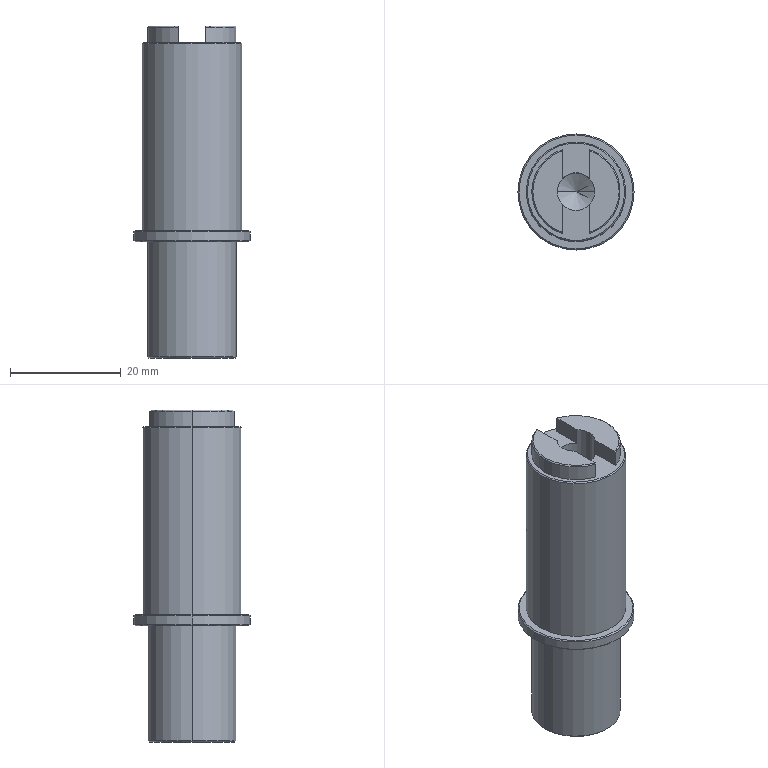Part | SolidWorks | features ICE 4, Chamfer 1, Extrusion 1, HoleWzd 1 | 1 solid | 34 faces | box 21 x 21 x 60 mm | volume 13278 mm3 | cone 13 | cylinder 11 | plane 10 | commonest cylinder face diameters 16 x5 6.8 x2 18 x2 21 x2
STEP:
#1=CARTESIAN_POINT('',(-7.8,0.,37.));
#2=VERTEX_POINT('',#1);
#3=CARTESIAN_POINT('',(-2.5,-7.389,37.));
#4=VERTEX_POINT('',#3);
#5=CARTESIAN_POINT('',(0.,0.,37.));
#6=DIRECTION('',(0.,0.,1.));
#7=DIRECTION('',(1.,0.,0.));
#8=AXIS2_PLACEMENT_3D('',#5,#6,#7);
#9=CIRCLE('',#8,7.8);
#10=EDGE_CURVE('',#2,#4,#9,.T.);
#11=ORIENTED_EDGE('',*,*,#10,.F.);
#12=CARTESIAN_POINT('',(-8.,0.,36.8));
#13=VERTEX_POINT('',#12);
#14=CARTESIAN_POINT('',(-7.8,0.,37.));
#15=DIRECTION('',(-0.7071,0.,-0.7071));
#16=VECTOR('',#15,1000.);
#17=LINE('',#14,#16);
#18=EDGE_CURVE('',#2,#13,#17,.T.);
#19=ORIENTED_EDGE('',*,*,#18,.T.);
#20=CARTESIAN_POINT('',(-2.5,-7.599,36.8));
#21=VERTEX_POINT('',#20);
#22=CARTESIAN_POINT('',(0.,0.,36.8));
#23=DIRECTION('',(0.,0.,-1.));
#24=DIRECTION('',(1.,0.,0.));
#25=AXIS2_PLACEMENT_3D('',#22,#23,#24);
#26=CIRCLE('',#25,8.);
#27=EDGE_CURVE('',#21,#13,#26,.T.);
#28=ORIENTED_EDGE('',*,*,#27,.F.);
#29=CARTESIAN_POINT('',(-2.5,-7.389,37.));
#30=CARTESIAN_POINT('',(-2.5,-7.459,36.933));
#31=CARTESIAN_POINT('',(-2.5,-7.529,36.867));
#32=CARTESIAN_POINT('',(-2.5,-7.599,36.8));
#33=B_SPLINE_CURVE_WITH_KNOTS('',3,(#29,#30,#31,#32),.UNSPECIFIED.,.F.,.F.,(4,4),(0.,0.0002906),.UNSPECIFIED.);
#34=EDGE_CURVE('',#4,#21,#33,.T.);
#35=ORIENTED_EDGE('',*,*,#34,.F.);
#36=EDGE_LOOP('',(#11,#19,#28,#35));
#37=FACE_OUTER_BOUND('',#36,.T.);
#38=CARTESIAN_POINT('',(0.,0.,37.));
#39=DIRECTION('',(0.,0.,-1.));
#40=DIRECTION('',(-1.,0.,0.));
#41=AXIS2_PLACEMENT_3D('',#38,#39,#40);
#42=CONICAL_SURFACE('',#41,7.8,0.7854);
#43=ADVANCED_FACE('',(#37),#42,.T.);
#44=CARTESIAN_POINT('',(8.8,0.,34.));
#45=VERTEX_POINT('',#44);
#46=CARTESIAN_POINT('',(-8.8,0.,34.));
#47=VERTEX_POINT('',#46);
#48=CARTESIAN_POINT('',(0.,0.,34.));
#49=DIRECTION('',(0.,0.,1.));
#50=DIRECTION('',(1.,0.,0.));
#51=AXIS2_PLACEMENT_3D('',#48,#49,#50);
#52=CIRCLE('',#51,8.8);
#53=EDGE_CURVE('',#45,#47,#52,.T.);
#54=ORIENTED_EDGE('',*,*,#53,.F.);
#55=CARTESIAN_POINT('',(9.,0.,33.8));
#56=VERTEX_POINT('',#55);
#57=CARTESIAN_POINT('',(8.8,0.,34.));
#58=DIRECTION('',(0.7071,0.,-0.7071));
#59=VECTOR('',#58,1000.);
#60=LINE('',#57,#59);
#61=EDGE_CURVE('',#45,#56,#60,.T.);
#62=ORIENTED_EDGE('',*,*,#61,.T.);
#63=CARTESIAN_POINT('',(-9.,0.,33.8));
#64=VERTEX_POINT('',#63);
#65=CARTESIAN_POINT('',(0.,0.,33.8));
#66=DIRECTION('',(0.,0.,-1.));
#67=DIRECTION('',(1.,0.,0.));
#68=AXIS2_PLACEMENT_3D('',#65,#66,#67);
#69=CIRCLE('',#68,9.);
#70=EDGE_CURVE('',#64,#56,#69,.T.);
#71=ORIENTED_EDGE('',*,*,#70,.F.);
#72=CARTESIAN_POINT('',(-8.8,0.,34.));
#73=DIRECTION('',(-0.7071,0.,-0.7071));
#74=VECTOR('',#73,1000.);
#75=LINE('',#72,#74);
#76=EDGE_CURVE('',#47,#64,#75,.T.);
#77=ORIENTED_EDGE('',*,*,#76,.F.);
#78=EDGE_LOOP('',(#54,#62,#71,#77));
#79=FACE_OUTER_BOUND('',#78,.T.);
#80=CARTESIAN_POINT('',(0.,0.,34.));
#81=DIRECTION('',(0.,0.,-1.));
#82=DIRECTION('',(-1.,0.,0.));
#83=AXIS2_PLACEMENT_3D('',#80,#81,#82);
#84=CONICAL_SURFACE('',#83,8.8,0.7854);
#85=ADVANCED_FACE('',(#79),#84,.T.);
#86=CARTESIAN_POINT('',(10.3,0.,0.));
#87=VERTEX_POINT('',#86);
#88=CARTESIAN_POINT('',(-10.3,0.,0.));
#89=VERTEX_POINT('',#88);
#90=CARTESIAN_POINT('',(0.,0.,0.));
#91=DIRECTION('',(0.,0.,1.));
#92=DIRECTION('',(-1.,0.,0.));
#93=AXIS2_PLACEMENT_3D('',#90,#91,#92);
#94=CIRCLE('',#93,10.3);
#95=EDGE_CURVE('',#87,#89,#94,.T.);
#96=ORIENTED_EDGE('',*,*,#95,.F.);
#97=CARTESIAN_POINT('',(10.5,0.,-0.2));
#98=VERTEX_POINT('',#97);
#99=CARTESIAN_POINT('',(10.5,0.,-0.2));
#100=DIRECTION('',(0.7071,0.,-0.7071));
#101=VECTOR('',#100,1000.);
#102=LINE('',#99,#101);
#103=EDGE_CURVE('',#87,#98,#102,.T.);
#104=ORIENTED_EDGE('',*,*,#103,.T.);
#105=CARTESIAN_POINT('',(-10.5,0.,-0.2));
#106=VERTEX_POINT('',#105);
#107=CARTESIAN_POINT('',(0.,0.,-0.2));
#108=DIRECTION('',(0.,0.,-1.));
#109=DIRECTION('',(-1.,0.,0.));
#110=AXIS2_PLACEMENT_3D('',#107,#108,#109);
#111=CIRCLE('',#110,10.5);
#112=EDGE_CURVE('',#106,#98,#111,.T.);
#113=ORIENTED_EDGE('',*,*,#112,.F.);
#114=CARTESIAN_POINT('',(-10.5,0.,-0.2));
#115=DIRECTION('',(-0.7071,0.,-0.7071));
#116=VECTOR('',#115,1000.);
#117=LINE('',#114,#116);
#118=EDGE_CURVE('',#89,#106,#117,.T.);
#119=ORIENTED_EDGE('',*,*,#118,.F.);
#120=EDGE_LOOP('',(#96,#104,#113,#119));
#121=FACE_OUTER_BOUND('',#120,.T.);
#122=CARTESIAN_POINT('',(0.,0.,-0.2));
#123=DIRECTION('',(0.,0.,-1.));
#124=DIRECTION('',(-1.,0.,0.));
#125=AXIS2_PLACEMENT_3D('',#122,#123,#124);
#126=CONICAL_SURFACE('',#125,10.5,0.7854);
#127=ADVANCED_FACE('',(#121),#126,.T.);
#128=CARTESIAN_POINT('',(-10.3,0.,-2.));
#129=VERTEX_POINT('',#128);
#130=CARTESIAN_POINT('',(10.3,0.,-2.));
#131=VERTEX_POINT('',#130);
#132=CARTESIAN_POINT('',(0.,0.,-2.));
#133=DIRECTION('',(0.,0.,-1.));
#134=DIRECTION('',(-1.,0.,0.));
#135=AXIS2_PLACEMENT_3D('',#132,#133,#134);
#136=CIRCLE('',#135,10.3);
#137=EDGE_CURVE('',#129,#131,#136,.T.);
#138=ORIENTED_EDGE('',*,*,#137,.F.);
#139=CARTESIAN_POINT('',(-10.5,0.,-1.8));
#140=VERTEX_POINT('',#139);
#141=CARTESIAN_POINT('',(-10.3,0.,-2.));
#142=DIRECTION('',(-0.7071,0.,0.7071));
#143=VECTOR('',#142,1000.);
#144=LINE('',#141,#143);
#145=EDGE_CURVE('',#129,#140,#144,.T.);
#146=ORIENTED_EDGE('',*,*,#145,.T.);
#147=CARTESIAN_POINT('',(10.5,0.,-1.8));
#148=VERTEX_POINT('',#147);
#149=CARTESIAN_POINT('',(0.,0.,-1.8));
#150=DIRECTION('',(0.,0.,1.));
#151=DIRECTION('',(-1.,0.,0.));
#152=AXIS2_PLACEMENT_3D('',#149,#150,#151);
#153=CIRCLE('',#152,10.5);
#154=EDGE_CURVE('',#148,#140,#153,.T.);
#155=ORIENTED_EDGE('',*,*,#154,.F.);
#156=CARTESIAN_POINT('',(10.3,0.,-2.));
#157=DIRECTION('',(0.7071,0.,0.7071));
#158=VECTOR('',#157,1000.);
#159=LINE('',#156,#158);
#160=EDGE_CURVE('',#131,#148,#159,.T.);
#161=ORIENTED_EDGE('',*,*,#160,.F.);
#162=EDGE_LOOP('',(#138,#146,#155,#161));
#163=FACE_OUTER_BOUND('',#162,.T.);
#164=CARTESIAN_POINT('',(0.,0.,-2.));
#165=DIRECTION('',(0.,0.,1.));
#166=DIRECTION('',(1.,0.,0.));
#167=AXIS2_PLACEMENT_3D('',#164,#165,#166);
#168=CONICAL_SURFACE('',#167,10.3,0.7854);
#169=ADVANCED_FACE('',(#163),#168,.T.);
#170=CARTESIAN_POINT('',(-7.8,0.,-23.));
#171=VERTEX_POINT('',#170);
#172=CARTESIAN_POINT('',(7.8,0.,-23.));
#173=VERTEX_POINT('',#172);
#174=CARTESIAN_POINT('',(0.,0.,-23.));
#175=DIRECTION('',(0.,0.,-1.));
#176=DIRECTION('',(-1.,0.,0.));
#177=AXIS2_PLACEMENT_3D('',#174,#175,#176);
#178=CIRCLE('',#177,7.8);
#179=EDGE_CURVE('',#171,#173,#178,.T.);
#180=ORIENTED_EDGE('',*,*,#179,.F.);
#181=CARTESIAN_POINT('',(-8.,0.,-22.8));
#182=VERTEX_POINT('',#181);
#183=CARTESIAN_POINT('',(-7.8,0.,-23.));
#184=DIRECTION('',(-0.7071,0.,0.7071));
#185=VECTOR('',#184,1000.);
#186=LINE('',#183,#185);
#187=EDGE_CURVE('',#171,#182,#186,.T.);
#188=ORIENTED_EDGE('',*,*,#187,.T.);
#189=CARTESIAN_POINT('',(8.,0.,-22.8));
#190=VERTEX_POINT('',#189);
#191=CARTESIAN_POINT('',(0.,0.,-22.8));
#192=DIRECTION('',(0.,0.,1.));
#193=DIRECTION('',(-1.,0.,0.));
#194=AXIS2_PLACEMENT_3D('',#191,#192,#193);
#195=CIRCLE('',#194,8.);
#196=EDGE_CURVE('',#190,#182,#195,.T.);
#197=ORIENTED_EDGE('',*,*,#196,.F.);
#198=CARTESIAN_POINT('',(7.8,0.,-23.));
#199=DIRECTION('',(0.7071,0.,0.7071));
#200=VECTOR('',#199,1000.);
#201=LINE('',#198,#200);
#202=EDGE_CURVE('',#173,#190,#201,.T.);
#203=ORIENTED_EDGE('',*,*,#202,.F.);
#204=EDGE_LOOP('',(#180,#188,#197,#203));
#205=FACE_OUTER_BOUND('',#204,.T.);
#206=CARTESIAN_POINT('',(0.,0.,-23.));
#207=DIRECTION('',(0.,0.,1.));
#208=DIRECTION('',(1.,0.,0.));
#209=AXIS2_PLACEMENT_3D('',#206,#207,#208);
#210=CONICAL_SURFACE('',#209,7.8,0.7854);
#211=ADVANCED_FACE('',(#205),#210,.T.);
#212=CARTESIAN_POINT('',(0.,0.,15.207));
#213=VERTEX_POINT('',#212);
#214=CARTESIAN_POINT('',(3.4,0.,17.25));
#215=VERTEX_POINT('',#214);
#216=CARTESIAN_POINT('',(3.4,0.,17.25));
#217=DIRECTION('',(0.8572,0.,0.515));
#218=VECTOR('',#217,1000.);
#219=LINE('',#216,#218);
#220=EDGE_CURVE('',#213,#215,#219,.T.);
#221=ORIENTED_EDGE('',*,*,#220,.F.);
#222=CARTESIAN_POINT('',(-3.4,0.,17.25));
#223=VERTEX_POINT('',#222);
#224=CARTESIAN_POINT('',(-3.4,0.,17.25));
#225=DIRECTION('',(-0.8572,0.,0.515));
#226=VECTOR('',#225,1000.);
#227=LINE('',#224,#226);
#228=EDGE_CURVE('',#213,#223,#227,.T.);
#229=ORIENTED_EDGE('',*,*,#228,.T.);
#230=CARTESIAN_POINT('',(0.,0.,17.25));
#231=DIRECTION('',(0.,0.,1.));
#232=DIRECTION('',(1.,0.,0.));
#233=AXIS2_PLACEMENT_3D('',#230,#231,#232);
#234=CIRCLE('',#233,3.4);
#235=EDGE_CURVE('',#223,#215,#234,.T.);
#236=ORIENTED_EDGE('',*,*,#235,.T.);
#237=EDGE_LOOP('',(#221,#229,#236));
#238=FACE_OUTER_BOUND('',#237,.T.);
#239=CARTESIAN_POINT('',(0.,0.,17.25));
#240=DIRECTION('',(0.,0.,1.));
#241=DIRECTION('',(1.,0.,0.));
#242=AXIS2_PLACEMENT_3D('',#239,#240,#241);
#243=CONICAL_SURFACE('',#242,3.4,1.03);
#244=ADVANCED_FACE('',(#238),#243,.F.);
#245=ORIENTED_EDGE('',*,*,#235,.F.);
#246=CARTESIAN_POINT('',(-3.4,0.,37.));
#247=VERTEX_POINT('',#246);
#248=CARTESIAN_POINT('',(-3.4,0.,37.));
#249=DIRECTION('',(0.,0.,1.));
#250=VECTOR('',#249,1000.);
#251=LINE('',#248,#250);
#252=EDGE_CURVE('',#223,#247,#251,.T.);
#253=ORIENTED_EDGE('',*,*,#252,.T.);
#254=CARTESIAN_POINT('',(-2.5,-2.304,37.));
#255=VERTEX_POINT('',#254);
#256=CARTESIAN_POINT('',(0.,0.,37.));
#257=DIRECTION('',(0.,0.,1.));
#258=DIRECTION('',(1.,0.,0.));
#259=AXIS2_PLACEMENT_3D('',#256,#257,#258);
#260=CIRCLE('',#259,3.4);
#261=EDGE_CURVE('',#247,#255,#260,.T.);
#262=ORIENTED_EDGE('',*,*,#261,.T.);
#263=CARTESIAN_POINT('',(-2.5,-2.304,34.));
#264=VERTEX_POINT('',#263);
#265=CARTESIAN_POINT('',(-2.5,-2.304,37.));
#266=DIRECTION('',(0.,0.,1.));
#267=VECTOR('',#266,1000.);
#268=LINE('',#265,#267);
#269=EDGE_CURVE('',#264,#255,#268,.T.);
#270=ORIENTED_EDGE('',*,*,#269,.F.);
#271=CARTESIAN_POINT('',(2.5,-2.304,34.));
#272=VERTEX_POINT('',#271);
#273=CARTESIAN_POINT('',(0.,0.,34.));
#274=DIRECTION('',(0.,0.,1.));
#275=DIRECTION('',(1.,0.,0.));
#276=AXIS2_PLACEMENT_3D('',#273,#274,#275);
#277=CIRCLE('',#276,3.4);
#278=EDGE_CURVE('',#264,#272,#277,.T.);
#279=ORIENTED_EDGE('',*,*,#278,.T.);
#280=CARTESIAN_POINT('',(2.5,-2.304,37.));
#281=VERTEX_POINT('',#280);
#282=CARTESIAN_POINT('',(2.5,-2.304,37.));
#283=DIRECTION('',(0.,0.,-1.));
#284=VECTOR('',#283,1000.);
#285=LINE('',#282,#284);
#286=EDGE_CURVE('',#281,#272,#285,.T.);
#287=ORIENTED_EDGE('',*,*,#286,.F.);
#288=CARTESIAN_POINT('',(3.4,0.,37.));
#289=VERTEX_POINT('',#288);
#290=CARTESIAN_POINT('',(0.,0.,37.));
#291=DIRECTION('',(0.,0.,1.));
#292=DIRECTION('',(1.,0.,0.));
#293=AXIS2_PLACEMENT_3D('',#290,#291,#292);
#294=CIRCLE('',#293,3.4);
#295=EDGE_CURVE('',#281,#289,#294,.T.);
#296=ORIENTED_EDGE('',*,*,#295,.T.);
#297=CARTESIAN_POINT('',(3.4,0.,37.));
#298=DIRECTION('',(0.,0.,1.));
#299=VECTOR('',#298,1000.);
#300=LINE('',#297,#299);
#301=EDGE_CURVE('',#215,#289,#300,.T.);
#302=ORIENTED_EDGE('',*,*,#301,.F.);
#303=EDGE_LOOP('',(#245,#253,#262,#270,#279,#287,#296,#302));
#304=FACE_OUTER_BOUND('',#303,.T.);
#305=CARTESIAN_POINT('',(0.,0.,37.));
#306=DIRECTION('',(0.,0.,1.));
#307=DIRECTION('',(1.,0.,0.));
#308=AXIS2_PLACEMENT_3D('',#305,#306,#307);
#309=CYLINDRICAL_SURFACE('',#308,3.4);
#310=ADVANCED_FACE('',(#304),#309,.F.);
#311=ORIENTED_EDGE('',*,*,#196,.T.);
#312=CARTESIAN_POINT('',(-8.,0.,-2.));
#313=VERTEX_POINT('',#312);
#314=CARTESIAN_POINT('',(-8.,0.,-23.));
#315=DIRECTION('',(0.,0.,1.));
#316=VECTOR('',#315,1000.);
#317=LINE('',#314,#316);
#318=EDGE_CURVE('',#182,#313,#317,.T.);
#319=ORIENTED_EDGE('',*,*,#318,.T.);
#320=CARTESIAN_POINT('',(8.,0.,-2.));
#321=VERTEX_POINT('',#320);
#322=CARTESIAN_POINT('',(0.,0.,-2.));
#323=DIRECTION('',(0.,0.,-1.));
#324=DIRECTION('',(-1.,0.,0.));
#325=AXIS2_PLACEMENT_3D('',#322,#323,#324);
#326=CIRCLE('',#325,8.);
#327=EDGE_CURVE('',#313,#321,#326,.T.);
#328=ORIENTED_EDGE('',*,*,#327,.T.);
#329=CARTESIAN_POINT('',(8.,0.,-23.));
#330=DIRECTION('',(0.,0.,1.));
#331=VECTOR('',#330,1000.);
#332=LINE('',#329,#331);
#333=EDGE_CURVE('',#190,#321,#332,.T.);
#334=ORIENTED_EDGE('',*,*,#333,.F.);
#335=EDGE_LOOP('',(#311,#319,#328,#334));
#336=FACE_OUTER_BOUND('',#335,.T.);
#337=CARTESIAN_POINT('',(0.,0.,-23.));
#338=DIRECTION('',(0.,0.,1.));
#339=DIRECTION('',(1.,0.,0.));
#340=AXIS2_PLACEMENT_3D('',#337,#338,#339);
#341=CYLINDRICAL_SURFACE('',#340,8.);
#342=ADVANCED_FACE('',(#336),#341,.T.);
#343=ORIENTED_EDGE('',*,*,#154,.T.);
#344=CARTESIAN_POINT('',(-10.5,0.,-2.));
#345=DIRECTION('',(0.,0.,1.));
#346=VECTOR('',#345,1000.);
#347=LINE('',#344,#346);
#348=EDGE_CURVE('',#140,#106,#347,.T.);
#349=ORIENTED_EDGE('',*,*,#348,.T.);
#350=ORIENTED_EDGE('',*,*,#112,.T.);
#351=CARTESIAN_POINT('',(10.5,0.,-2.));
#352=DIRECTION('',(0.,0.,1.));
#353=VECTOR('',#352,1000.);
#354=LINE('',#351,#353);
#355=EDGE_CURVE('',#148,#98,#354,.T.);
#356=ORIENTED_EDGE('',*,*,#355,.F.);
#357=EDGE_LOOP('',(#343,#349,#350,#356));
#358=FACE_OUTER_BOUND('',#357,.T.);
#359=CARTESIAN_POINT('',(0.,0.,-2.));
#360=DIRECTION('',(0.,0.,1.));
#361=DIRECTION('',(1.,0.,0.));
#362=AXIS2_PLACEMENT_3D('',#359,#360,#361);
#363=CYLINDRICAL_SURFACE('',#362,10.5);
#364=ADVANCED_FACE('',(#358),#363,.T.);
#365=ORIENTED_EDGE('',*,*,#70,.T.);
#366=CARTESIAN_POINT('',(9.,0.,0.));
#367=VERTEX_POINT('',#366);
#368=CARTESIAN_POINT('',(9.,0.,34.));
#369=DIRECTION('',(0.,0.,-1.));
#370=VECTOR('',#369,1000.);
#371=LINE('',#368,#370);
#372=EDGE_CURVE('',#56,#367,#371,.T.);
#373=ORIENTED_EDGE('',*,*,#372,.T.);
#374=CARTESIAN_POINT('',(-9.,0.,0.));
#375=VERTEX_POINT('',#374);
#376=CARTESIAN_POINT('',(0.,0.,0.));
#377=DIRECTION('',(0.,0.,-1.));
#378=DIRECTION('',(-1.,0.,0.));
#379=AXIS2_PLACEMENT_3D('',#376,#377,#378);
#380=CIRCLE('',#379,9.);
#381=EDGE_CURVE('',#375,#367,#380,.T.);
#382=ORIENTED_EDGE('',*,*,#381,.F.);
#383=CARTESIAN_POINT('',(-9.,0.,34.));
#384=DIRECTION('',(0.,0.,-1.));
#385=VECTOR('',#384,1000.);
#386=LINE('',#383,#385);
#387=EDGE_CURVE('',#64,#375,#386,.T.);
#388=ORIENTED_EDGE('',*,*,#387,.F.);
#389=EDGE_LOOP('',(#365,#373,#382,#388));
#390=FACE_OUTER_BOUND('',#389,.T.);
#391=CARTESIAN_POINT('',(0.,0.,34.));
#392=DIRECTION('',(0.,0.,-1.));
#393=DIRECTION('',(-1.,0.,0.));
#394=AXIS2_PLACEMENT_3D('',#391,#392,#393);
#395=CYLINDRICAL_SURFACE('',#394,9.);
#396=ADVANCED_FACE('',(#390),#395,.T.);
#397=ORIENTED_EDGE('',*,*,#27,.T.);
#398=CARTESIAN_POINT('',(-8.,0.,34.));
#399=VERTEX_POINT('',#398);
#400=CARTESIAN_POINT('',(-8.,0.,37.));
#401=DIRECTION('',(0.,0.,-1.));
#402=VECTOR('',#401,1000.);
#403=LINE('',#400,#402);
#404=EDGE_CURVE('',#13,#399,#403,.T.);
#405=ORIENTED_EDGE('',*,*,#404,.T.);
#406=CARTESIAN_POINT('',(-2.5,-7.599,34.));
#407=VERTEX_POINT('',#406);
#408=CARTESIAN_POINT('',(0.,0.,34.));
#409=DIRECTION('',(0.,0.,1.));
#410=DIRECTION('',(1.,0.,0.));
#411=AXIS2_PLACEMENT_3D('',#408,#409,#410);
#412=CIRCLE('',#411,8.);
#413=EDGE_CURVE('',#399,#407,#412,.T.);
#414=ORIENTED_EDGE('',*,*,#413,.T.);
#415=CARTESIAN_POINT('',(-2.5,-7.599,37.));
#416=DIRECTION('',(0.,0.,1.));
#417=VECTOR('',#416,1000.);
#418=LINE('',#415,#417);
#419=EDGE_CURVE('',#407,#21,#418,.T.);
#420=ORIENTED_EDGE('',*,*,#419,.T.);
#421=EDGE_LOOP('',(#397,#405,#414,#420));
#422=FACE_OUTER_BOUND('',#421,.T.);
#423=CARTESIAN_POINT('',(0.,0.,37.));
#424=DIRECTION('',(0.,0.,-1.));
#425=DIRECTION('',(-1.,0.,0.));
#426=AXIS2_PLACEMENT_3D('',#423,#424,#425);
#427=CYLINDRICAL_SURFACE('',#426,8.);
#428=ADVANCED_FACE('',(#422),#427,.T.);
#429=CARTESIAN_POINT('',(-2.5,0.,37.));
#430=DIRECTION('',(0.,-1.,0.));
#431=VECTOR('',#430,1000.);
#432=LINE('',#429,#431);
#433=EDGE_CURVE('',#255,#4,#432,.T.);
#434=ORIENTED_EDGE('',*,*,#433,.T.);
#435=ORIENTED_EDGE('',*,*,#34,.T.);
#436=ORIENTED_EDGE('',*,*,#419,.F.);
#437=CARTESIAN_POINT('',(-2.5,-14.294,34.));
#438=DIRECTION('',(0.,-1.,0.));
#439=VECTOR('',#438,1000.);
#440=LINE('',#437,#439);
#441=EDGE_CURVE('',#264,#407,#440,.T.);
#442=ORIENTED_EDGE('',*,*,#441,.F.);
#443=ORIENTED_EDGE('',*,*,#269,.T.);
#444=EDGE_LOOP('',(#434,#435,#436,#442,#443));
#445=FACE_OUTER_BOUND('',#444,.T.);
#446=CARTESIAN_POINT('',(-2.5,-14.294,34.));
#447=DIRECTION('',(-1.,0.,0.));
#448=DIRECTION('',(0.,0.,1.));
#449=AXIS2_PLACEMENT_3D('',#446,#447,#448);
#450=PLANE('',#449);
#451=ADVANCED_FACE('',(#445),#450,.F.);
#452=CARTESIAN_POINT('',(2.5,2.304,37.));
#453=VERTEX_POINT('',#452);
#454=CARTESIAN_POINT('',(2.5,7.389,37.));
#455=VERTEX_POINT('',#454);
#456=CARTESIAN_POINT('',(2.5,0.,37.));
#457=DIRECTION('',(0.,1.,0.));
#458=VECTOR('',#457,1000.);
#459=LINE('',#456,#458);
#460=EDGE_CURVE('',#453,#455,#459,.T.);
#461=ORIENTED_EDGE('',*,*,#460,.T.);
#462=CARTESIAN_POINT('',(2.5,7.599,36.8));
#463=VERTEX_POINT('',#462);
#464=CARTESIAN_POINT('',(2.5,7.389,37.));
#465=CARTESIAN_POINT('',(2.5,7.459,36.933));
#466=CARTESIAN_POINT('',(2.5,7.529,36.867));
#467=CARTESIAN_POINT('',(2.5,7.599,36.8));
#468=B_SPLINE_CURVE_WITH_KNOTS('',3,(#464,#465,#466,#467),.UNSPECIFIED.,.F.,.F.,(4,4),(0.,0.0002906),.UNSPECIFIED.);
#469=EDGE_CURVE('',#455,#463,#468,.T.);
#470=ORIENTED_EDGE('',*,*,#469,.T.);
#471=CARTESIAN_POINT('',(2.5,7.599,34.));
#472=VERTEX_POINT('',#471);
#473=CARTESIAN_POINT('',(2.5,7.599,37.));
#474=DIRECTION('',(0.,0.,1.));
#475=VECTOR('',#474,1000.);
#476=LINE('',#473,#475);
#477=EDGE_CURVE('',#472,#463,#476,.T.);
#478=ORIENTED_EDGE('',*,*,#477,.F.);
#479=CARTESIAN_POINT('',(2.5,2.304,34.));
#480=VERTEX_POINT('',#479);
#481=CARTESIAN_POINT('',(2.5,-14.294,34.));
#482=DIRECTION('',(0.,1.,0.));
#483=VECTOR('',#482,1000.);
#484=LINE('',#481,#483);
#485=EDGE_CURVE('',#480,#472,#484,.T.);
#486=ORIENTED_EDGE('',*,*,#485,.F.);
#487=CARTESIAN_POINT('',(2.5,2.304,37.));
#488=DIRECTION('',(0.,0.,1.));
#489=VECTOR('',#488,1000.);
#490=LINE('',#487,#489);
#491=EDGE_CURVE('',#480,#453,#490,.T.);
#492=ORIENTED_EDGE('',*,*,#491,.T.);
#493=EDGE_LOOP('',(#461,#470,#478,#486,#492));
#494=FACE_OUTER_BOUND('',#493,.T.);
#495=CARTESIAN_POINT('',(2.5,-14.294,34.));
#496=DIRECTION('',(1.,0.,0.));
#497=DIRECTION('',(0.,0.,-1.));
#498=AXIS2_PLACEMENT_3D('',#495,#496,#497);
#499=PLANE('',#498);
#500=ADVANCED_FACE('',(#494),#499,.F.);
#501=ORIENTED_EDGE('',*,*,#404,.F.);
#502=CARTESIAN_POINT('',(-2.5,7.599,36.8));
#503=VERTEX_POINT('',#502);
#504=CARTESIAN_POINT('',(0.,0.,36.8));
#505=DIRECTION('',(0.,0.,-1.));
#506=DIRECTION('',(1.,0.,0.));
#507=AXIS2_PLACEMENT_3D('',#504,#505,#506);
#508=CIRCLE('',#507,8.);
#509=EDGE_CURVE('',#13,#503,#508,.T.);
#510=ORIENTED_EDGE('',*,*,#509,.T.);
#511=CARTESIAN_POINT('',(-2.5,7.599,34.));
#512=VERTEX_POINT('',#511);
#513=CARTESIAN_POINT('',(-2.5,7.599,37.));
#514=DIRECTION('',(0.,0.,-1.));
#515=VECTOR('',#514,1000.);
#516=LINE('',#513,#515);
#517=EDGE_CURVE('',#503,#512,#516,.T.);
#518=ORIENTED_EDGE('',*,*,#517,.T.);
#519=CARTESIAN_POINT('',(0.,0.,34.));
#520=DIRECTION('',(0.,0.,1.));
#521=DIRECTION('',(1.,0.,0.));
#522=AXIS2_PLACEMENT_3D('',#519,#520,#521);
#523=CIRCLE('',#522,8.);
#524=EDGE_CURVE('',#512,#399,#523,.T.);
#525=ORIENTED_EDGE('',*,*,#524,.T.);
#526=EDGE_LOOP('',(#501,#510,#518,#525));
#527=FACE_OUTER_BOUND('',#526,.T.);
#528=CARTESIAN_POINT('',(0.,0.,37.));
#529=DIRECTION('',(0.,0.,-1.));
#530=DIRECTION('',(-1.,0.,0.));
#531=AXIS2_PLACEMENT_3D('',#528,#529,#530);
#532=CYLINDRICAL_SURFACE('',#531,8.);
#533=ADVANCED_FACE('',(#527),#532,.T.);
#534=CARTESIAN_POINT('',(-2.5,7.389,37.));
#535=VERTEX_POINT('',#534);
#536=CARTESIAN_POINT('',(-2.5,2.304,37.));
#537=VERTEX_POINT('',#536);
#538=CARTESIAN_POINT('',(-2.5,0.,37.));
#539=DIRECTION('',(0.,-1.,0.));
#540=VECTOR('',#539,1000.);
#541=LINE('',#538,#540);
#542=EDGE_CURVE('',#535,#537,#541,.T.);
#543=ORIENTED_EDGE('',*,*,#542,.F.);
#544=CARTESIAN_POINT('',(0.,0.,37.));
#545=DIRECTION('',(0.,0.,1.));
#546=DIRECTION('',(1.,0.,0.));
#547=AXIS2_PLACEMENT_3D('',#544,#545,#546);
#548=CIRCLE('',#547,7.8);
#549=EDGE_CURVE('',#535,#2,#548,.T.);
#550=ORIENTED_EDGE('',*,*,#549,.T.);
#551=ORIENTED_EDGE('',*,*,#10,.T.);
#552=ORIENTED_EDGE('',*,*,#433,.F.);
#553=ORIENTED_EDGE('',*,*,#261,.F.);
#554=CARTESIAN_POINT('',(0.,0.,37.));
#555=DIRECTION('',(0.,0.,1.));
#556=DIRECTION('',(1.,0.,0.));
#557=AXIS2_PLACEMENT_3D('',#554,#555,#556);
#558=CIRCLE('',#557,3.4);
#559=EDGE_CURVE('',#537,#247,#558,.T.);
#560=ORIENTED_EDGE('',*,*,#559,.F.);
#561=EDGE_LOOP('',(#543,#550,#551,#552,#553,#560));
#562=FACE_OUTER_BOUND('',#561,.T.);
#563=CARTESIAN_POINT('',(0.,0.,37.));
#564=DIRECTION('',(0.,0.,1.));
#565=DIRECTION('',(1.,0.,0.));
#566=AXIS2_PLACEMENT_3D('',#563,#564,#565);
#567=PLANE('',#566);
#568=ADVANCED_FACE('',(#562),#567,.T.);
#569=CARTESIAN_POINT('',(0.,0.,-2.));
#570=DIRECTION('',(0.,0.,-1.));
#571=DIRECTION('',(-1.,0.,0.));
#572=AXIS2_PLACEMENT_3D('',#569,#570,#571);
#573=CIRCLE('',#572,10.3);
#574=EDGE_CURVE('',#131,#129,#573,.T.);
#575=ORIENTED_EDGE('',*,*,#574,.T.);
#576=ORIENTED_EDGE('',*,*,#137,.T.);
#577=EDGE_LOOP('',(#575,#576));
#578=FACE_OUTER_BOUND('',#577,.T.);
#579=CARTESIAN_POINT('',(0.,0.,-2.));
#580=DIRECTION('',(0.,0.,-1.));
#581=DIRECTION('',(-1.,0.,0.));
#582=AXIS2_PLACEMENT_3D('',#579,#580,#581);
#583=CIRCLE('',#582,8.);
#584=EDGE_CURVE('',#321,#313,#583,.T.);
#585=ORIENTED_EDGE('',*,*,#584,.F.);
#586=ORIENTED_EDGE('',*,*,#327,.F.);
#587=EDGE_LOOP('',(#585,#586));
#588=FACE_BOUND('',#587,.T.);
#589=CARTESIAN_POINT('',(0.,0.,-2.));
#590=DIRECTION('',(0.,0.,-1.));
#591=DIRECTION('',(-1.,0.,0.));
#592=AXIS2_PLACEMENT_3D('',#589,#590,#591);
#593=PLANE('',#592);
#594=ADVANCED_FACE('',(#578,#588),#593,.T.);
#595=CARTESIAN_POINT('',(0.,0.,34.));
#596=DIRECTION('',(0.,0.,1.));
#597=DIRECTION('',(1.,0.,0.));
#598=AXIS2_PLACEMENT_3D('',#595,#596,#597);
#599=CIRCLE('',#598,8.8);
#600=EDGE_CURVE('',#47,#45,#599,.T.);
#601=ORIENTED_EDGE('',*,*,#600,.T.);
#602=ORIENTED_EDGE('',*,*,#53,.T.);
#603=EDGE_LOOP('',(#601,#602));
#604=FACE_OUTER_BOUND('',#603,.T.);
#605=CARTESIAN_POINT('',(-2.5,2.304,34.));
#606=VERTEX_POINT('',#605);
#607=CARTESIAN_POINT('',(0.,0.,34.));
#608=DIRECTION('',(0.,0.,1.));
#609=DIRECTION('',(1.,0.,0.));
#610=AXIS2_PLACEMENT_3D('',#607,#608,#609);
#611=CIRCLE('',#610,3.4);
#612=EDGE_CURVE('',#480,#606,#611,.T.);
#613=ORIENTED_EDGE('',*,*,#612,.F.);
#614=ORIENTED_EDGE('',*,*,#485,.T.);
#615=CARTESIAN_POINT('',(2.5,-7.599,34.));
#616=VERTEX_POINT('',#615);
#617=CARTESIAN_POINT('',(0.,0.,34.));
#618=DIRECTION('',(0.,0.,1.));
#619=DIRECTION('',(1.,0.,0.));
#620=AXIS2_PLACEMENT_3D('',#617,#618,#619);
#621=CIRCLE('',#620,8.);
#622=EDGE_CURVE('',#616,#472,#621,.T.);
#623=ORIENTED_EDGE('',*,*,#622,.F.);
#624=CARTESIAN_POINT('',(2.5,-14.294,34.));
#625=DIRECTION('',(0.,1.,0.));
#626=VECTOR('',#625,1000.);
#627=LINE('',#624,#626);
#628=EDGE_CURVE('',#616,#272,#627,.T.);
#629=ORIENTED_EDGE('',*,*,#628,.T.);
#630=ORIENTED_EDGE('',*,*,#278,.F.);
#631=ORIENTED_EDGE('',*,*,#441,.T.);
#632=ORIENTED_EDGE('',*,*,#413,.F.);
#633=ORIENTED_EDGE('',*,*,#524,.F.);
#634=CARTESIAN_POINT('',(-2.5,-14.294,34.));
#635=DIRECTION('',(0.,-1.,0.));
#636=VECTOR('',#635,1000.);
#637=LINE('',#634,#636);
#638=EDGE_CURVE('',#512,#606,#637,.T.);
#639=ORIENTED_EDGE('',*,*,#638,.T.);
#640=EDGE_LOOP('',(#613,#614,#623,#629,#630,#631,#632,#633,#639));
#641=FACE_BOUND('',#640,.T.);
#642=CARTESIAN_POINT('',(0.,0.,34.));
#643=DIRECTION('',(0.,0.,1.));
#644=DIRECTION('',(1.,0.,0.));
#645=AXIS2_PLACEMENT_3D('',#642,#643,#644);
#646=PLANE('',#645);
#647=ADVANCED_FACE('',(#604,#641),#646,.T.);
#648=ORIENTED_EDGE('',*,*,#372,.F.);
#649=CARTESIAN_POINT('',(0.,0.,33.8));
#650=DIRECTION('',(0.,0.,-1.));
#651=DIRECTION('',(1.,0.,0.));
#652=AXIS2_PLACEMENT_3D('',#649,#650,#651);
#653=CIRCLE('',#652,9.);
#654=EDGE_CURVE('',#56,#64,#653,.T.);
#655=ORIENTED_EDGE('',*,*,#654,.T.);
#656=ORIENTED_EDGE('',*,*,#387,.T.);
#657=CARTESIAN_POINT('',(0.,0.,0.));
#658=DIRECTION('',(0.,0.,-1.));
#659=DIRECTION('',(-1.,0.,0.));
#660=AXIS2_PLACEMENT_3D('',#657,#658,#659);
#661=CIRCLE('',#660,9.);
#662=EDGE_CURVE('',#367,#375,#661,.T.);
#663=ORIENTED_EDGE('',*,*,#662,.F.);
#664=EDGE_LOOP('',(#648,#655,#656,#663));
#665=FACE_OUTER_BOUND('',#664,.T.);
#666=CARTESIAN_POINT('',(0.,0.,34.));
#667=DIRECTION('',(0.,0.,-1.));
#668=DIRECTION('',(-1.,0.,0.));
#669=AXIS2_PLACEMENT_3D('',#666,#667,#668);
#670=CYLINDRICAL_SURFACE('',#669,9.);
#671=ADVANCED_FACE('',(#665),#670,.T.);
#672=ORIENTED_EDGE('',*,*,#477,.T.);
#673=CARTESIAN_POINT('',(2.5,-7.599,36.8));
#674=VERTEX_POINT('',#673);
#675=CARTESIAN_POINT('',(0.,0.,36.8));
#676=DIRECTION('',(0.,0.,-1.));
#677=DIRECTION('',(1.,0.,0.));
#678=AXIS2_PLACEMENT_3D('',#675,#676,#677);
#679=CIRCLE('',#678,8.);
#680=EDGE_CURVE('',#463,#674,#679,.T.);
#681=ORIENTED_EDGE('',*,*,#680,.T.);
#682=CARTESIAN_POINT('',(2.5,-7.599,37.));
#683=DIRECTION('',(0.,0.,-1.));
#684=VECTOR('',#683,1000.);
#685=LINE('',#682,#684);
#686=EDGE_CURVE('',#674,#616,#685,.T.);
#687=ORIENTED_EDGE('',*,*,#686,.T.);
#688=ORIENTED_EDGE('',*,*,#622,.T.);
#689=EDGE_LOOP('',(#672,#681,#687,#688));
#690=FACE_OUTER_BOUND('',#689,.T.);
#691=CARTESIAN_POINT('',(0.,0.,37.));
#692=DIRECTION('',(0.,0.,-1.));
#693=DIRECTION('',(-1.,0.,0.));
#694=AXIS2_PLACEMENT_3D('',#691,#692,#693);
#695=CYLINDRICAL_SURFACE('',#694,8.);
#696=ADVANCED_FACE('',(#690),#695,.T.);
#697=CARTESIAN_POINT('',(2.5,-7.389,37.));
#698=VERTEX_POINT('',#697);
#699=CARTESIAN_POINT('',(2.5,0.,37.));
#700=DIRECTION('',(0.,1.,0.));
#701=VECTOR('',#700,1000.);
#702=LINE('',#699,#701);
#703=EDGE_CURVE('',#698,#281,#702,.T.);
#704=ORIENTED_EDGE('',*,*,#703,.F.);
#705=CARTESIAN_POINT('',(0.,0.,37.));
#706=DIRECTION('',(0.,0.,1.));
#707=DIRECTION('',(1.,0.,0.));
#708=AXIS2_PLACEMENT_3D('',#705,#706,#707);
#709=CIRCLE('',#708,7.8);
#710=EDGE_CURVE('',#698,#455,#709,.T.);
#711=ORIENTED_EDGE('',*,*,#710,.T.);
#712=ORIENTED_EDGE('',*,*,#460,.F.);
#713=CARTESIAN_POINT('',(0.,0.,37.));
#714=DIRECTION('',(0.,0.,1.));
#715=DIRECTION('',(1.,0.,0.));
#716=AXIS2_PLACEMENT_3D('',#713,#714,#715);
#717=CIRCLE('',#716,3.4);
#718=EDGE_CURVE('',#289,#453,#717,.T.);
#719=ORIENTED_EDGE('',*,*,#718,.F.);
#720=ORIENTED_EDGE('',*,*,#295,.F.);
#721=EDGE_LOOP('',(#704,#711,#712,#719,#720));
#722=FACE_OUTER_BOUND('',#721,.T.);
#723=CARTESIAN_POINT('',(0.,0.,37.));
#724=DIRECTION('',(0.,0.,1.));
#725=DIRECTION('',(1.,0.,0.));
#726=AXIS2_PLACEMENT_3D('',#723,#724,#725);
#727=PLANE('',#726);
#728=ADVANCED_FACE('',(#722),#727,.T.);
#729=CARTESIAN_POINT('',(0.,0.,0.));
#730=DIRECTION('',(0.,0.,1.));
#731=DIRECTION('',(-1.,0.,0.));
#732=AXIS2_PLACEMENT_3D('',#729,#730,#731);
#733=CIRCLE('',#732,10.3);
#734=EDGE_CURVE('',#89,#87,#733,.T.);
#735=ORIENTED_EDGE('',*,*,#734,.T.);
#736=ORIENTED_EDGE('',*,*,#95,.T.);
#737=EDGE_LOOP('',(#735,#736));
#738=FACE_OUTER_BOUND('',#737,.T.);
#739=ORIENTED_EDGE('',*,*,#381,.T.);
#740=ORIENTED_EDGE('',*,*,#662,.T.);
#741=EDGE_LOOP('',(#739,#740));
#742=FACE_BOUND('',#741,.T.);
#743=CARTESIAN_POINT('',(0.,0.,0.));
#744=DIRECTION('',(0.,0.,-1.));
#745=DIRECTION('',(-1.,0.,0.));
#746=AXIS2_PLACEMENT_3D('',#743,#744,#745);
#747=PLANE('',#746);
#748=ADVANCED_FACE('',(#738,#742),#747,.F.);
#749=ORIENTED_EDGE('',*,*,#348,.F.);
#750=CARTESIAN_POINT('',(0.,0.,-1.8));
#751=DIRECTION('',(0.,0.,1.));
#752=DIRECTION('',(-1.,0.,0.));
#753=AXIS2_PLACEMENT_3D('',#750,#751,#752);
#754=CIRCLE('',#753,10.5);
#755=EDGE_CURVE('',#140,#148,#754,.T.);
#756=ORIENTED_EDGE('',*,*,#755,.T.);
#757=ORIENTED_EDGE('',*,*,#355,.T.);
#758=CARTESIAN_POINT('',(0.,0.,-0.2));
#759=DIRECTION('',(0.,0.,-1.));
#760=DIRECTION('',(-1.,0.,0.));
#761=AXIS2_PLACEMENT_3D('',#758,#759,#760);
#762=CIRCLE('',#761,10.5);
#763=EDGE_CURVE('',#98,#106,#762,.T.);
#764=ORIENTED_EDGE('',*,*,#763,.T.);
#765=EDGE_LOOP('',(#749,#756,#757,#764));
#766=FACE_OUTER_BOUND('',#765,.T.);
#767=CARTESIAN_POINT('',(0.,0.,-2.));
#768=DIRECTION('',(0.,0.,1.));
#769=DIRECTION('',(1.,0.,0.));
#770=AXIS2_PLACEMENT_3D('',#767,#768,#769);
#771=CYLINDRICAL_SURFACE('',#770,10.5);
#772=ADVANCED_FACE('',(#766),#771,.T.);
#773=ORIENTED_EDGE('',*,*,#318,.F.);
#774=CARTESIAN_POINT('',(0.,0.,-22.8));
#775=DIRECTION('',(0.,0.,1.));
#776=DIRECTION('',(-1.,0.,0.));
#777=AXIS2_PLACEMENT_3D('',#774,#775,#776);
#778=CIRCLE('',#777,8.);
#779=EDGE_CURVE('',#182,#190,#778,.T.);
#780=ORIENTED_EDGE('',*,*,#779,.T.);
#781=ORIENTED_EDGE('',*,*,#333,.T.);
#782=ORIENTED_EDGE('',*,*,#584,.T.);
#783=EDGE_LOOP('',(#773,#780,#781,#782));
#784=FACE_OUTER_BOUND('',#783,.T.);
#785=CARTESIAN_POINT('',(0.,0.,-23.));
#786=DIRECTION('',(0.,0.,1.));
#787=DIRECTION('',(1.,0.,0.));
#788=AXIS2_PLACEMENT_3D('',#785,#786,#787);
#789=CYLINDRICAL_SURFACE('',#788,8.);
#790=ADVANCED_FACE('',(#784),#789,.T.);
#791=CARTESIAN_POINT('',(0.,0.,-23.));
#792=DIRECTION('',(0.,0.,-1.));
#793=DIRECTION('',(-1.,0.,0.));
#794=AXIS2_PLACEMENT_3D('',#791,#792,#793);
#795=CIRCLE('',#794,7.8);
#796=EDGE_CURVE('',#173,#171,#795,.T.);
#797=ORIENTED_EDGE('',*,*,#796,.T.);
#798=ORIENTED_EDGE('',*,*,#179,.T.);
#799=EDGE_LOOP('',(#797,#798));
#800=FACE_OUTER_BOUND('',#799,.T.);
#801=CARTESIAN_POINT('',(0.,0.,-23.));
#802=DIRECTION('',(0.,0.,-1.));
#803=DIRECTION('',(-1.,0.,0.));
#804=AXIS2_PLACEMENT_3D('',#801,#802,#803);
#805=PLANE('',#804);
#806=ADVANCED_FACE('',(#800),#805,.T.);
#807=ORIENTED_EDGE('',*,*,#517,.F.);
#808=CARTESIAN_POINT('',(-2.5,7.599,36.8));
#809=CARTESIAN_POINT('',(-2.5,7.529,36.867));
#810=CARTESIAN_POINT('',(-2.5,7.459,36.933));
#811=CARTESIAN_POINT('',(-2.5,7.389,37.));
#812=B_SPLINE_CURVE_WITH_KNOTS('',3,(#808,#809,#810,#811),.UNSPECIFIED.,.F.,.F.,(4,4),(0.,0.0002906),.UNSPECIFIED.);
#813=EDGE_CURVE('',#503,#535,#812,.T.);
#814=ORIENTED_EDGE('',*,*,#813,.T.);
#815=ORIENTED_EDGE('',*,*,#542,.T.);
#816=CARTESIAN_POINT('',(-2.5,2.304,37.));
#817=DIRECTION('',(0.,0.,-1.));
#818=VECTOR('',#817,1000.);
#819=LINE('',#816,#818);
#820=EDGE_CURVE('',#537,#606,#819,.T.);
#821=ORIENTED_EDGE('',*,*,#820,.T.);
#822=ORIENTED_EDGE('',*,*,#638,.F.);
#823=EDGE_LOOP('',(#807,#814,#815,#821,#822));
#824=FACE_OUTER_BOUND('',#823,.T.);
#825=CARTESIAN_POINT('',(-2.5,-14.294,34.));
#826=DIRECTION('',(-1.,0.,0.));
#827=DIRECTION('',(0.,0.,1.));
#828=AXIS2_PLACEMENT_3D('',#825,#826,#827);
#829=PLANE('',#828);
#830=ADVANCED_FACE('',(#824),#829,.F.);
#831=ORIENTED_EDGE('',*,*,#686,.F.);
#832=CARTESIAN_POINT('',(2.5,-7.599,36.8));
#833=CARTESIAN_POINT('',(2.5,-7.529,36.867));
#834=CARTESIAN_POINT('',(2.5,-7.459,36.933));
#835=CARTESIAN_POINT('',(2.5,-7.389,37.));
#836=B_SPLINE_CURVE_WITH_KNOTS('',3,(#832,#833,#834,#835),.UNSPECIFIED.,.F.,.F.,(4,4),(0.,0.0002906),.UNSPECIFIED.);
#837=EDGE_CURVE('',#674,#698,#836,.T.);
#838=ORIENTED_EDGE('',*,*,#837,.T.);
#839=ORIENTED_EDGE('',*,*,#703,.T.);
#840=ORIENTED_EDGE('',*,*,#286,.T.);
#841=ORIENTED_EDGE('',*,*,#628,.F.);
#842=EDGE_LOOP('',(#831,#838,#839,#840,#841));
#843=FACE_OUTER_BOUND('',#842,.T.);
#844=CARTESIAN_POINT('',(2.5,-14.294,34.));
#845=DIRECTION('',(1.,0.,0.));
#846=DIRECTION('',(0.,0.,-1.));
#847=AXIS2_PLACEMENT_3D('',#844,#845,#846);
#848=PLANE('',#847);
#849=ADVANCED_FACE('',(#843),#848,.F.);
#850=ORIENTED_EDGE('',*,*,#252,.F.);
#851=CARTESIAN_POINT('',(0.,0.,17.25));
#852=DIRECTION('',(0.,0.,1.));
#853=DIRECTION('',(1.,0.,0.));
#854=AXIS2_PLACEMENT_3D('',#851,#852,#853);
#855=CIRCLE('',#854,3.4);
#856=EDGE_CURVE('',#215,#223,#855,.T.);
#857=ORIENTED_EDGE('',*,*,#856,.F.);
#858=ORIENTED_EDGE('',*,*,#301,.T.);
#859=ORIENTED_EDGE('',*,*,#718,.T.);
#860=ORIENTED_EDGE('',*,*,#491,.F.);
#861=ORIENTED_EDGE('',*,*,#612,.T.);
#862=ORIENTED_EDGE('',*,*,#820,.F.);
#863=ORIENTED_EDGE('',*,*,#559,.T.);
#864=EDGE_LOOP('',(#850,#857,#858,#859,#860,#861,#862,#863));
#865=FACE_OUTER_BOUND('',#864,.T.);
#866=CARTESIAN_POINT('',(0.,0.,37.));
#867=DIRECTION('',(0.,0.,1.));
#868=DIRECTION('',(1.,0.,0.));
#869=AXIS2_PLACEMENT_3D('',#866,#867,#868);
#870=CYLINDRICAL_SURFACE('',#869,3.4);
#871=ADVANCED_FACE('',(#865),#870,.F.);
#872=ORIENTED_EDGE('',*,*,#228,.F.);
#873=ORIENTED_EDGE('',*,*,#220,.T.);
#874=ORIENTED_EDGE('',*,*,#856,.T.);
#875=EDGE_LOOP('',(#872,#873,#874));
#876=FACE_OUTER_BOUND('',#875,.T.);
#877=CARTESIAN_POINT('',(0.,0.,17.25));
#878=DIRECTION('',(0.,0.,1.));
#879=DIRECTION('',(1.,0.,0.));
#880=AXIS2_PLACEMENT_3D('',#877,#878,#879);
#881=CONICAL_SURFACE('',#880,3.4,1.03);
#882=ADVANCED_FACE('',(#876),#881,.F.);
#883=ORIENTED_EDGE('',*,*,#187,.F.);
#884=ORIENTED_EDGE('',*,*,#796,.F.);
#885=ORIENTED_EDGE('',*,*,#202,.T.);
#886=ORIENTED_EDGE('',*,*,#779,.F.);
#887=EDGE_LOOP('',(#883,#884,#885,#886));
#888=FACE_OUTER_BOUND('',#887,.T.);
#889=CARTESIAN_POINT('',(0.,0.,-23.));
#890=DIRECTION('',(0.,0.,1.));
#891=DIRECTION('',(1.,0.,0.));
#892=AXIS2_PLACEMENT_3D('',#889,#890,#891);
#893=CONICAL_SURFACE('',#892,7.8,0.7854);
#894=ADVANCED_FACE('',(#888),#893,.T.);
#895=ORIENTED_EDGE('',*,*,#145,.F.);
#896=ORIENTED_EDGE('',*,*,#574,.F.);
#897=ORIENTED_EDGE('',*,*,#160,.T.);
#898=ORIENTED_EDGE('',*,*,#755,.F.);
#899=EDGE_LOOP('',(#895,#896,#897,#898));
#900=FACE_OUTER_BOUND('',#899,.T.);
#901=CARTESIAN_POINT('',(0.,0.,-2.));
#902=DIRECTION('',(0.,0.,1.));
#903=DIRECTION('',(1.,0.,0.));
#904=AXIS2_PLACEMENT_3D('',#901,#902,#903);
#905=CONICAL_SURFACE('',#904,10.3,0.7854);
#906=ADVANCED_FACE('',(#900),#905,.T.);
#907=ORIENTED_EDGE('',*,*,#103,.F.);
#908=ORIENTED_EDGE('',*,*,#734,.F.);
#909=ORIENTED_EDGE('',*,*,#118,.T.);
#910=ORIENTED_EDGE('',*,*,#763,.F.);
#911=EDGE_LOOP('',(#907,#908,#909,#910));
#912=FACE_OUTER_BOUND('',#911,.T.);
#913=CARTESIAN_POINT('',(0.,0.,-0.2));
#914=DIRECTION('',(0.,0.,-1.));
#915=DIRECTION('',(-1.,0.,0.));
#916=AXIS2_PLACEMENT_3D('',#913,#914,#915);
#917=CONICAL_SURFACE('',#916,10.5,0.7854);
#918=ADVANCED_FACE('',(#912),#917,.T.);
#919=ORIENTED_EDGE('',*,*,#61,.F.);
#920=ORIENTED_EDGE('',*,*,#600,.F.);
#921=ORIENTED_EDGE('',*,*,#76,.T.);
#922=ORIENTED_EDGE('',*,*,#654,.F.);
#923=EDGE_LOOP('',(#919,#920,#921,#922));
#924=FACE_OUTER_BOUND('',#923,.T.);
#925=CARTESIAN_POINT('',(0.,0.,34.));
#926=DIRECTION('',(0.,0.,-1.));
#927=DIRECTION('',(-1.,0.,0.));
#928=AXIS2_PLACEMENT_3D('',#925,#926,#927);
#929=CONICAL_SURFACE('',#928,8.8,0.7854);
#930=ADVANCED_FACE('',(#924),#929,.T.);
#931=ORIENTED_EDGE('',*,*,#837,.F.);
#932=ORIENTED_EDGE('',*,*,#680,.F.);
#933=ORIENTED_EDGE('',*,*,#469,.F.);
#934=ORIENTED_EDGE('',*,*,#710,.F.);
#935=EDGE_LOOP('',(#931,#932,#933,#934));
#936=FACE_OUTER_BOUND('',#935,.T.);
#937=CARTESIAN_POINT('',(0.,0.,37.));
#938=DIRECTION('',(0.,0.,-1.));
#939=DIRECTION('',(-1.,0.,0.));
#940=AXIS2_PLACEMENT_3D('',#937,#938,#939);
#941=CONICAL_SURFACE('',#940,7.8,0.7854);
#942=ADVANCED_FACE('',(#936),#941,.T.);
#943=ORIENTED_EDGE('',*,*,#18,.F.);
#944=ORIENTED_EDGE('',*,*,#549,.F.);
#945=ORIENTED_EDGE('',*,*,#813,.F.);
#946=ORIENTED_EDGE('',*,*,#509,.F.);
#947=EDGE_LOOP('',(#943,#944,#945,#946));
#948=FACE_OUTER_BOUND('',#947,.T.);
#949=CARTESIAN_POINT('',(0.,0.,37.));
#950=DIRECTION('',(0.,0.,-1.));
#951=DIRECTION('',(-1.,0.,0.));
#952=AXIS2_PLACEMENT_3D('',#949,#950,#951);
#953=CONICAL_SURFACE('',#952,7.8,0.7854);
#954=ADVANCED_FACE('',(#948),#953,.T.);
#955=CLOSED_SHELL('',(#43,#85,#127,#169,#211,#244,#310,#342,#364,#396,#428,#451,#500,#533,#568,#594,#647,#671,#696,#728,#748,#772,#790,#806,#830,#849,#871,#882,#894,#906,#918,#930,#942,#954));
#956=MANIFOLD_SOLID_BREP('',#955);
#957=CARTESIAN_POINT('',(0.,0.,0.));
#958=DIRECTION('',(0.,0.,1.));
#959=DIRECTION('',(1.,0.,0.));
#960=AXIS2_PLACEMENT_3D('',#957,#958,#959);
#961=(LENGTH_UNIT()NAMED_UNIT(*)SI_UNIT(.MILLI.,.METRE.));
#962=UNCERTAINTY_MEASURE_WITH_UNIT(LENGTH_MEASURE(0.00001),#961,'','');
#963=(NAMED_UNIT(*)PLANE_ANGLE_UNIT()SI_UNIT($,.RADIAN.));
#964=(NAMED_UNIT(*)SI_UNIT($,.STERADIAN.)SOLID_ANGLE_UNIT());
#965=(GEOMETRIC_REPRESENTATION_CONTEXT(3)GLOBAL_UNCERTAINTY_ASSIGNED_CONTEXT((#962))GLOBAL_UNIT_ASSIGNED_CONTEXT((#961,#963,#964))REPRESENTATION_CONTEXT('',''));
#966=ADVANCED_BREP_SHAPE_REPRESENTATION('',(#956,#960),#965);